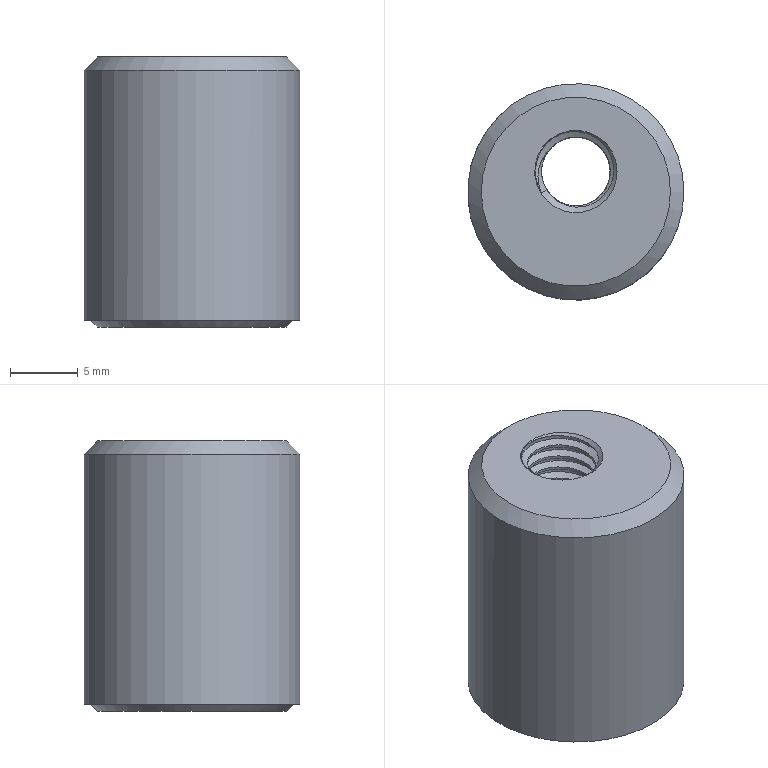Part | NX | features solid 2 | 1 solid | 21 faces | box 16.01 x 16 x 20.007 mm | volume 3058 mm3 | plane 10 | cone 5 | cylinder 4 | spline 2 | commonest cylinder face diameters 5.1 x1 6 x1 9 x1 16 x1
STEP:
#1=CARTESIAN_POINT('',(524.742,-196.458,-46.502));
#2=VERTEX_POINT('',#1);
#3=CARTESIAN_POINT('',(520.,-201.2,-46.5));
#4=VERTEX_POINT('',#3);
#5=CARTESIAN_POINT('',(522.371,-198.829,-46.501));
#6=DIRECTION('',(-0.7071,-0.7071,0.0003672));
#7=VECTOR('',#6,1000.);
#8=LINE('',#5,#7);
#9=EDGE_CURVE('',#2,#4,#8,.T.);
#10=ORIENTED_EDGE('',*,*,#9,.F.);
#11=CARTESIAN_POINT('',(523.742,-196.458,-46.502));
#12=VERTEX_POINT('',#11);
#13=CARTESIAN_POINT('',(524.242,-196.458,-46.502));
#14=DIRECTION('',(-1.,0.,0.0005193));
#15=VECTOR('',#14,1000.);
#16=LINE('',#13,#15);
#17=EDGE_CURVE('',#2,#12,#16,.T.);
#18=ORIENTED_EDGE('',*,*,#17,.T.);
#19=CARTESIAN_POINT('',(520.,-200.2,-46.5));
#20=VERTEX_POINT('',#19);
#21=CARTESIAN_POINT('',(521.871,-198.329,-46.501));
#22=DIRECTION('',(-0.7071,-0.7071,0.0003672));
#23=VECTOR('',#22,1000.);
#24=LINE('',#21,#23);
#25=EDGE_CURVE('',#12,#20,#24,.T.);
#26=ORIENTED_EDGE('',*,*,#25,.T.);
#27=CARTESIAN_POINT('',(516.154,-196.354,-46.498));
#28=VERTEX_POINT('',#27);
#29=CARTESIAN_POINT('',(517.827,-198.027,-46.499));
#30=DIRECTION('',(-0.7071,0.7071,0.0003672));
#31=VECTOR('',#30,1000.);
#32=LINE('',#29,#31);
#33=EDGE_CURVE('',#20,#28,#32,.T.);
#34=ORIENTED_EDGE('',*,*,#33,.T.);
#35=CARTESIAN_POINT('',(515.154,-196.354,-46.497));
#36=VERTEX_POINT('',#35);
#37=CARTESIAN_POINT('',(515.154,-196.354,-46.497));
#38=DIRECTION('',(1.,0.,-0.0005193));
#39=VECTOR('',#38,1000.);
#40=LINE('',#37,#39);
#41=EDGE_CURVE('',#36,#28,#40,.T.);
#42=ORIENTED_EDGE('',*,*,#41,.F.);
#43=CARTESIAN_POINT('',(517.577,-198.777,-46.499));
#44=DIRECTION('',(-0.7071,0.7071,0.0003672));
#45=VECTOR('',#44,1000.);
#46=LINE('',#43,#45);
#47=EDGE_CURVE('',#4,#36,#46,.T.);
#48=ORIENTED_EDGE('',*,*,#47,.F.);
#49=EDGE_LOOP('',(#10,#18,#26,#34,#42,#48));
#50=FACE_BOUND('',#49,.T.);
#51=CARTESIAN_POINT('',(524.5,-193.5,-46.502));
#52=VERTEX_POINT('',#51);
#53=CARTESIAN_POINT('',(520.,-193.5,-46.5));
#54=DIRECTION('',(0.0005193,0.,1.));
#55=DIRECTION('',(1.,0.,-0.0005193));
#56=AXIS2_PLACEMENT_3D('',#53,#54,#55);
#57=CIRCLE('',#56,4.5);
#58=EDGE_CURVE('',#52,#52,#57,.T.);
#59=ORIENTED_EDGE('',*,*,#58,.T.);
#60=EDGE_LOOP('',(#59));
#61=FACE_BOUND('',#60,.T.);
#62=CARTESIAN_POINT('',(526.5,-195.,-46.503));
#63=VERTEX_POINT('',#62);
#64=CARTESIAN_POINT('',(520.,-195.,-46.5));
#65=DIRECTION('',(0.0005193,0.,1.));
#66=DIRECTION('',(1.,0.,-0.0005193));
#67=AXIS2_PLACEMENT_3D('',#64,#65,#66);
#68=CIRCLE('',#67,6.5);
#69=EDGE_CURVE('',#63,#63,#68,.T.);
#70=ORIENTED_EDGE('',*,*,#69,.F.);
#71=EDGE_LOOP('',(#70));
#72=FACE_BOUND('',#71,.T.);
#73=CARTESIAN_POINT('',(520.,-195.,-46.5));
#74=DIRECTION('',(-0.0005193,0.,-1.));
#75=DIRECTION('',(1.,0.,-0.0005193));
#76=AXIS2_PLACEMENT_3D('',#73,#74,#75);
#77=PLANE('',#76);
#78=ADVANCED_FACE('',(#50,#61,#72),#77,.T.);
#79=CARTESIAN_POINT('',(512.5,-195.,-46.496));
#80=VERTEX_POINT('',#79);
#81=CARTESIAN_POINT('',(520.,-195.,-46.5));
#82=DIRECTION('',(-0.0005193,0.,-1.));
#83=DIRECTION('',(-1.,0.,0.0005193));
#84=AXIS2_PLACEMENT_3D('',#81,#82,#83);
#85=CIRCLE('',#84,7.5);
#86=EDGE_CURVE('',#80,#80,#85,.T.);
#87=ORIENTED_EDGE('',*,*,#86,.F.);
#88=EDGE_LOOP('',(#87));
#89=FACE_BOUND('',#88,.T.);
#90=CARTESIAN_POINT('',(528.,-195.,-46.504));
#91=VERTEX_POINT('',#90);
#92=CARTESIAN_POINT('',(520.,-195.,-46.5));
#93=DIRECTION('',(0.0005193,0.,1.));
#94=DIRECTION('',(1.,0.,-0.0005193));
#95=AXIS2_PLACEMENT_3D('',#92,#93,#94);
#96=CIRCLE('',#95,8.);
#97=EDGE_CURVE('',#91,#91,#96,.T.);
#98=ORIENTED_EDGE('',*,*,#97,.F.);
#99=EDGE_LOOP('',(#98));
#100=FACE_BOUND('',#99,.T.);
#101=CARTESIAN_POINT('',(520.,-195.,-46.5));
#102=DIRECTION('',(-0.0005193,0.,-1.));
#103=DIRECTION('',(1.,0.,-0.0005193));
#104=AXIS2_PLACEMENT_3D('',#101,#102,#103);
#105=PLANE('',#104);
#106=ADVANCED_FACE('',(#89,#100),#105,.T.);
#107=CARTESIAN_POINT('',(527.01,-195.,-27.004));
#108=VERTEX_POINT('',#107);
#109=CARTESIAN_POINT('',(520.01,-195.,-27.));
#110=DIRECTION('',(0.0005193,0.,1.));
#111=DIRECTION('',(1.,0.,-0.0005193));
#112=AXIS2_PLACEMENT_3D('',#109,#110,#111);
#113=CIRCLE('',#112,7.);
#114=EDGE_CURVE('',#108,#108,#113,.T.);
#115=ORIENTED_EDGE('',*,*,#114,.T.);
#116=EDGE_LOOP('',(#115));
#117=FACE_BOUND('',#116,.T.);
#118=CARTESIAN_POINT('',(523.06,-193.5,-27.002));
#119=VERTEX_POINT('',#118);
#120=CARTESIAN_POINT('',(520.01,-193.5,-27.));
#121=DIRECTION('',(-0.0005193,0.,-1.));
#122=DIRECTION('',(1.,0.,-0.0005193));
#123=AXIS2_PLACEMENT_3D('',#120,#121,#122);
#124=CIRCLE('',#123,3.05);
#125=EDGE_CURVE('',#119,#119,#124,.T.);
#126=ORIENTED_EDGE('',*,*,#125,.T.);
#127=EDGE_LOOP('',(#126));
#128=FACE_BOUND('',#127,.T.);
#129=CARTESIAN_POINT('',(520.01,-195.,-27.));
#130=DIRECTION('',(0.0005193,0.,1.));
#131=DIRECTION('',(-1.,0.,0.0005193));
#132=AXIS2_PLACEMENT_3D('',#129,#130,#131);
#133=PLANE('',#132);
#134=ADVANCED_FACE('',(#117,#128),#133,.T.);
#135=CARTESIAN_POINT('',(528.01,-195.,-28.004));
#136=VERTEX_POINT('',#135);
#137=CARTESIAN_POINT('',(520.01,-195.,-28.));
#138=DIRECTION('',(-0.0005193,0.,-1.));
#139=DIRECTION('',(1.,0.,-0.0005193));
#140=AXIS2_PLACEMENT_3D('',#137,#138,#139);
#141=CIRCLE('',#140,8.);
#142=EDGE_CURVE('',#136,#136,#141,.T.);
#143=ORIENTED_EDGE('',*,*,#142,.T.);
#144=EDGE_LOOP('',(#143));
#145=FACE_BOUND('',#144,.T.);
#146=ORIENTED_EDGE('',*,*,#97,.T.);
#147=EDGE_LOOP('',(#146));
#148=FACE_BOUND('',#147,.T.);
#149=CARTESIAN_POINT('',(520.,-195.,-46.5));
#150=DIRECTION('',(0.0005193,0.,1.));
#151=DIRECTION('',(-1.,0.,0.0005193));
#152=AXIS2_PLACEMENT_3D('',#149,#150,#151);
#153=CYLINDRICAL_SURFACE('',#152,8.);
#154=ADVANCED_FACE('',(#145,#148),#153,.T.);
#155=CARTESIAN_POINT('',(522.07,-194.996,-37.001));
#156=VERTEX_POINT('',#155);
#157=CARTESIAN_POINT('',(522.07,-192.004,-37.001));
#158=VERTEX_POINT('',#157);
#159=CARTESIAN_POINT('',(520.005,-193.5,-37.));
#160=DIRECTION('',(0.0005193,0.,1.));
#161=DIRECTION('',(1.,0.,-0.0005193));
#162=AXIS2_PLACEMENT_3D('',#159,#160,#161);
#163=CIRCLE('',#162,2.55);
#164=EDGE_CURVE('',#156,#158,#163,.T.);
#165=ORIENTED_EDGE('',*,*,#164,.F.);
#166=CARTESIAN_POINT('',(517.945,-192.004,-27.499));
#167=VERTEX_POINT('',#166);
#168=CARTESIAN_POINT('',(522.07,-194.996,-37.001));
#169=CARTESIAN_POINT('',(522.54,-194.348,-36.949));
#170=CARTESIAN_POINT('',(522.813,-192.619,-36.853));
#171=CARTESIAN_POINT('',(520.969,-190.713,-36.703));
#172=CARTESIAN_POINT('',(518.34,-191.069,-36.553));
#173=CARTESIAN_POINT('',(517.061,-193.388,-36.406));
#174=CARTESIAN_POINT('',(518.16,-195.798,-36.257));
#175=CARTESIAN_POINT('',(520.753,-196.351,-36.109));
#176=CARTESIAN_POINT('',(522.741,-194.597,-35.961));
#177=CARTESIAN_POINT('',(522.516,-191.957,-35.813));
#178=CARTESIAN_POINT('',(520.264,-190.564,-35.666));
#179=CARTESIAN_POINT('',(517.801,-191.544,-35.515));
#180=CARTESIAN_POINT('',(517.122,-194.107,-35.366));
#181=CARTESIAN_POINT('',(518.776,-196.178,-35.217));
#182=CARTESIAN_POINT('',(521.422,-196.084,-35.07));
#183=CARTESIAN_POINT('',(522.926,-193.902,-34.924));
#184=CARTESIAN_POINT('',(522.067,-191.393,-34.775));
#185=CARTESIAN_POINT('',(519.541,-190.59,-34.625));
#186=CARTESIAN_POINT('',(517.394,-192.138,-34.474));
#187=CARTESIAN_POINT('',(517.355,-194.788,-34.326));
#188=CARTESIAN_POINT('',(519.463,-196.397,-34.18));
#189=CARTESIAN_POINT('',(522.01,-195.661,-34.033));
#190=CARTESIAN_POINT('',(522.936,-193.181,-33.885));
#191=CARTESIAN_POINT('',(521.496,-190.957,-33.734));
#192=CARTESIAN_POINT('',(518.85,-190.789,-33.584));
#193=CARTESIAN_POINT('',(517.141,-192.816,-33.436));
#194=CARTESIAN_POINT('',(517.749,-195.393,-33.288));
#195=CARTESIAN_POINT('',(520.182,-196.442,-33.142));
#196=CARTESIAN_POINT('',(522.475,-195.112,-32.993));
#197=CARTESIAN_POINT('',(522.771,-192.477,-32.844));
#198=CARTESIAN_POINT('',(520.833,-190.671,-32.695));
#199=CARTESIAN_POINT('',(518.228,-191.151,-32.546));
#200=CARTESIAN_POINT('',(517.06,-193.531,-32.399));
#201=CARTESIAN_POINT('',(518.278,-195.886,-32.249));
#202=CARTESIAN_POINT('',(520.893,-196.311,-32.101));
#203=CARTESIAN_POINT('',(522.792,-194.465,-31.954));
#204=CARTESIAN_POINT('',(522.442,-191.837,-31.806));
#205=CARTESIAN_POINT('',(520.121,-190.555,-31.658));
#206=CARTESIAN_POINT('',(517.71,-191.655,-31.507));
#207=CARTESIAN_POINT('',(517.157,-194.244,-31.358));
#208=CARTESIAN_POINT('',(518.908,-196.234,-31.21));
#209=CARTESIAN_POINT('',(521.55,-196.012,-31.063));
#210=CARTESIAN_POINT('',(522.944,-193.757,-30.917));
#211=CARTESIAN_POINT('',(521.966,-191.297,-30.767));
#212=CARTESIAN_POINT('',(519.405,-190.615,-30.617));
#213=CARTESIAN_POINT('',(517.331,-192.267,-30.466));
#214=CARTESIAN_POINT('',(517.425,-194.917,-30.318));
#215=CARTESIAN_POINT('',(519.605,-196.419,-30.173));
#216=CARTESIAN_POINT('',(522.113,-195.564,-30.025));
#217=CARTESIAN_POINT('',(522.92,-193.038,-29.877));
#218=CARTESIAN_POINT('',(521.371,-190.886,-29.726));
#219=CARTESIAN_POINT('',(518.723,-190.849,-29.577));
#220=CARTESIAN_POINT('',(517.113,-192.953,-29.429));
#221=CARTESIAN_POINT('',(517.845,-195.502,-29.281));
#222=CARTESIAN_POINT('',(520.329,-196.43,-29.134));
#223=CARTESIAN_POINT('',(522.552,-194.99,-28.985));
#224=CARTESIAN_POINT('',(522.721,-192.346,-28.837));
#225=CARTESIAN_POINT('',(520.697,-190.634,-28.688));
#226=CARTESIAN_POINT('',(518.116,-191.241,-28.539));
#227=CARTESIAN_POINT('',(517.068,-193.674,-28.391));
#228=CARTESIAN_POINT('',(518.396,-195.966,-28.241));
#229=CARTESIAN_POINT('',(521.03,-196.265,-28.094));
#230=CARTESIAN_POINT('',(522.839,-194.327,-27.946));
#231=CARTESIAN_POINT('',(522.359,-191.72,-27.798));
#232=CARTESIAN_POINT('',(519.981,-190.556,-27.649));
#233=CARTESIAN_POINT('',(518.415,-191.356,-27.551));
#234=CARTESIAN_POINT('',(517.945,-192.004,-27.499));
#235=B_SPLINE_CURVE_WITH_KNOTS('',3,(#168,#169,#170,#171,#172,#173,#174,#175,#176,#177,#178,#179,#180,#181,#182,#183,#184,#185,#186,#187,#188,#189,#190,#191,#192,#193,#194,#195,#196,#197,#198,#199,#200,#201,#202,#203,#204,#205,#206,#207,#208,#209,#210,#211,#212,#213,#214,#215,#216,#217,#218,#219,#220,#221,#222,#223,#224,#225,#226,#227,#228,#229,#230,#231,#232,#233,#234),.UNSPECIFIED.,.F.,.F.,(4,1,1,1,1,1,1,1,1,1,1,1,1,1,1,1,1,1,1,1,1,1,1,1,1,1,1,1,1,1,1,1,1,1,1,1,1,1,1,1,1,1,1,1,1,1,1,1,1,1,1,1,1,1,1,1,1,1,1,1,1,1,1,1,4),(0.,0.002372,0.004743,0.007115,0.009486,0.01186,0.01423,0.0166,0.01897,0.02134,0.02372,0.02609,0.02846,0.03083,0.0332,0.03557,0.03795,0.04032,0.04269,0.04506,0.04743,0.0498,0.05217,0.05455,0.05692,0.05929,0.06166,0.06403,0.0664,0.06878,0.07115,0.07352,0.07589,0.07826,0.08063,0.083,0.08538,0.08775,0.09012,0.09249,0.09486,0.09723,0.09961,0.102,0.1043,0.1067,0.1091,0.1115,0.1138,0.1162,0.1186,0.1209,0.1233,0.1257,0.1281,0.1304,0.1328,0.1352,0.1376,0.1399,0.1423,0.1447,0.147,0.1494,0.1518),.UNSPECIFIED.);
#236=EDGE_CURVE('',#156,#167,#235,.T.);
#237=ORIENTED_EDGE('',*,*,#236,.T.);
#238=CARTESIAN_POINT('',(517.945,-194.996,-27.499));
#239=VERTEX_POINT('',#238);
#240=CARTESIAN_POINT('',(520.01,-193.5,-27.5));
#241=DIRECTION('',(0.0005193,0.,1.));
#242=DIRECTION('',(1.,0.,-0.0005193));
#243=AXIS2_PLACEMENT_3D('',#240,#241,#242);
#244=CIRCLE('',#243,2.55);
#245=EDGE_CURVE('',#167,#239,#244,.T.);
#246=ORIENTED_EDGE('',*,*,#245,.T.);
#247=CARTESIAN_POINT('',(517.945,-194.996,-27.499));
#248=CARTESIAN_POINT('',(517.476,-194.348,-27.551));
#249=CARTESIAN_POINT('',(517.202,-192.619,-27.647));
#250=CARTESIAN_POINT('',(519.047,-190.713,-27.797));
#251=CARTESIAN_POINT('',(521.675,-191.069,-27.947));
#252=CARTESIAN_POINT('',(522.954,-193.388,-28.094));
#253=CARTESIAN_POINT('',(521.855,-195.798,-28.243));
#254=CARTESIAN_POINT('',(519.263,-196.351,-28.391));
#255=CARTESIAN_POINT('',(517.274,-194.597,-28.539));
#256=CARTESIAN_POINT('',(517.499,-191.957,-28.687));
#257=CARTESIAN_POINT('',(519.751,-190.564,-28.834));
#258=CARTESIAN_POINT('',(522.214,-191.544,-28.985));
#259=CARTESIAN_POINT('',(522.894,-194.107,-29.134));
#260=CARTESIAN_POINT('',(521.239,-196.178,-29.283));
#261=CARTESIAN_POINT('',(518.593,-196.084,-29.43));
#262=CARTESIAN_POINT('',(517.089,-193.902,-29.576));
#263=CARTESIAN_POINT('',(517.948,-191.393,-29.725));
#264=CARTESIAN_POINT('',(520.474,-190.59,-29.875));
#265=CARTESIAN_POINT('',(522.622,-192.138,-30.026));
#266=CARTESIAN_POINT('',(522.66,-194.788,-30.174));
#267=CARTESIAN_POINT('',(520.552,-196.397,-30.32));
#268=CARTESIAN_POINT('',(518.005,-195.661,-30.467));
#269=CARTESIAN_POINT('',(517.079,-193.181,-30.615));
#270=CARTESIAN_POINT('',(518.519,-190.957,-30.766));
#271=CARTESIAN_POINT('',(521.165,-190.789,-30.916));
#272=CARTESIAN_POINT('',(522.875,-192.816,-31.064));
#273=CARTESIAN_POINT('',(522.266,-195.393,-31.212));
#274=CARTESIAN_POINT('',(519.834,-196.442,-31.358));
#275=CARTESIAN_POINT('',(517.54,-195.112,-31.507));
#276=CARTESIAN_POINT('',(517.244,-192.477,-31.656));
#277=CARTESIAN_POINT('',(519.182,-190.671,-31.805));
#278=CARTESIAN_POINT('',(521.787,-191.151,-31.954));
#279=CARTESIAN_POINT('',(522.955,-193.531,-32.101));
#280=CARTESIAN_POINT('',(521.738,-195.886,-32.251));
#281=CARTESIAN_POINT('',(519.122,-196.311,-32.399));
#282=CARTESIAN_POINT('',(517.223,-194.465,-32.546));
#283=CARTESIAN_POINT('',(517.573,-191.837,-32.694));
#284=CARTESIAN_POINT('',(519.894,-190.555,-32.842));
#285=CARTESIAN_POINT('',(522.305,-191.655,-32.993));
#286=CARTESIAN_POINT('',(522.858,-194.244,-33.142));
#287=CARTESIAN_POINT('',(521.108,-196.234,-33.29));
#288=CARTESIAN_POINT('',(518.465,-196.012,-33.437));
#289=CARTESIAN_POINT('',(517.071,-193.757,-33.583));
#290=CARTESIAN_POINT('',(518.05,-191.297,-33.733));
#291=CARTESIAN_POINT('',(520.61,-190.615,-33.883));
#292=CARTESIAN_POINT('',(522.684,-192.267,-34.034));
#293=CARTESIAN_POINT('',(522.591,-194.917,-34.182));
#294=CARTESIAN_POINT('',(520.41,-196.419,-34.327));
#295=CARTESIAN_POINT('',(517.902,-195.564,-34.475));
#296=CARTESIAN_POINT('',(517.095,-193.038,-34.623));
#297=CARTESIAN_POINT('',(518.645,-190.886,-34.774));
#298=CARTESIAN_POINT('',(521.292,-190.849,-34.923));
#299=CARTESIAN_POINT('',(522.902,-192.953,-35.071));
#300=CARTESIAN_POINT('',(522.17,-195.502,-35.219));
#301=CARTESIAN_POINT('',(519.686,-196.43,-35.366));
#302=CARTESIAN_POINT('',(517.464,-194.99,-35.515));
#303=CARTESIAN_POINT('',(517.294,-192.346,-35.663));
#304=CARTESIAN_POINT('',(519.318,-190.634,-35.812));
#305=CARTESIAN_POINT('',(521.899,-191.241,-35.961));
#306=CARTESIAN_POINT('',(522.947,-193.674,-36.109));
#307=CARTESIAN_POINT('',(521.62,-195.966,-36.259));
#308=CARTESIAN_POINT('',(518.985,-196.265,-36.406));
#309=CARTESIAN_POINT('',(517.176,-194.327,-36.554));
#310=CARTESIAN_POINT('',(517.656,-191.72,-36.702));
#311=CARTESIAN_POINT('',(520.035,-190.556,-36.851));
#312=CARTESIAN_POINT('',(521.601,-191.356,-36.949));
#313=CARTESIAN_POINT('',(522.07,-192.004,-37.001));
#314=B_SPLINE_CURVE_WITH_KNOTS('',3,(#247,#248,#249,#250,#251,#252,#253,#254,#255,#256,#257,#258,#259,#260,#261,#262,#263,#264,#265,#266,#267,#268,#269,#270,#271,#272,#273,#274,#275,#276,#277,#278,#279,#280,#281,#282,#283,#284,#285,#286,#287,#288,#289,#290,#291,#292,#293,#294,#295,#296,#297,#298,#299,#300,#301,#302,#303,#304,#305,#306,#307,#308,#309,#310,#311,#312,#313),.UNSPECIFIED.,.F.,.F.,(4,1,1,1,1,1,1,1,1,1,1,1,1,1,1,1,1,1,1,1,1,1,1,1,1,1,1,1,1,1,1,1,1,1,1,1,1,1,1,1,1,1,1,1,1,1,1,1,1,1,1,1,1,1,1,1,1,1,1,1,1,1,1,1,4),(0.,0.002372,0.004743,0.007115,0.009486,0.01186,0.01423,0.0166,0.01897,0.02134,0.02372,0.02609,0.02846,0.03083,0.0332,0.03557,0.03795,0.04032,0.04269,0.04506,0.04743,0.0498,0.05217,0.05455,0.05692,0.05929,0.06166,0.06403,0.0664,0.06878,0.07115,0.07352,0.07589,0.07826,0.08063,0.083,0.08538,0.08775,0.09012,0.09249,0.09486,0.09723,0.09961,0.102,0.1043,0.1067,0.1091,0.1115,0.1138,0.1162,0.1186,0.1209,0.1233,0.1257,0.1281,0.1304,0.1328,0.1352,0.1376,0.1399,0.1423,0.1447,0.147,0.1494,0.1518),.UNSPECIFIED.);
#315=EDGE_CURVE('',#239,#158,#314,.T.);
#316=ORIENTED_EDGE('',*,*,#315,.T.);
#317=EDGE_LOOP('',(#165,#237,#246,#316));
#318=FACE_BOUND('',#317,.T.);
#319=CARTESIAN_POINT('',(520.011,-193.5,-26.5));
#320=DIRECTION('',(0.0005193,0.,1.));
#321=DIRECTION('',(-1.,0.,0.0005193));
#322=AXIS2_PLACEMENT_3D('',#319,#320,#321);
#323=CYLINDRICAL_SURFACE('',#322,2.55);
#324=ADVANCED_FACE('',(#318),#323,.F.);
#325=CARTESIAN_POINT('',(518.102,-191.181,-36.999));
#326=VERTEX_POINT('',#325);
#327=CARTESIAN_POINT('',(518.102,-195.819,-36.999));
#328=VERTEX_POINT('',#327);
#329=CARTESIAN_POINT('',(520.005,-193.5,-37.));
#330=DIRECTION('',(0.0005193,0.,1.));
#331=DIRECTION('',(1.,0.,-0.0005193));
#332=AXIS2_PLACEMENT_3D('',#329,#330,#331);
#333=CIRCLE('',#332,3.);
#334=EDGE_CURVE('',#326,#328,#333,.T.);
#335=ORIENTED_EDGE('',*,*,#334,.T.);
#336=CARTESIAN_POINT('',(518.102,-195.819,-36.999));
#337=CARTESIAN_POINT('',(518.737,-196.246,-36.999));
#338=CARTESIAN_POINT('',(520.325,-196.591,-37.));
#339=CARTESIAN_POINT('',(521.693,-195.663,-37.001));
#340=CARTESIAN_POINT('',(522.07,-194.996,-37.001));
#341=B_SPLINE_CURVE_WITH_KNOTS('',3,(#336,#337,#338,#339,#340),.UNSPECIFIED.,.F.,.F.,(4,1,4),(0.,0.002262,0.004525),.UNSPECIFIED.);
#342=EDGE_CURVE('',#328,#156,#341,.T.);
#343=ORIENTED_EDGE('',*,*,#342,.T.);
#344=ORIENTED_EDGE('',*,*,#164,.T.);
#345=CARTESIAN_POINT('',(522.07,-192.004,-37.001));
#346=CARTESIAN_POINT('',(521.693,-191.338,-37.001));
#347=CARTESIAN_POINT('',(520.327,-190.409,-37.));
#348=CARTESIAN_POINT('',(518.737,-190.754,-36.999));
#349=CARTESIAN_POINT('',(518.102,-191.181,-36.999));
#350=B_SPLINE_CURVE_WITH_KNOTS('',3,(#345,#346,#347,#348,#349),.UNSPECIFIED.,.F.,.F.,(4,1,4),(0.,0.002264,0.004528),.UNSPECIFIED.);
#351=EDGE_CURVE('',#158,#326,#350,.T.);
#352=ORIENTED_EDGE('',*,*,#351,.T.);
#353=EDGE_LOOP('',(#335,#343,#344,#352));
#354=FACE_BOUND('',#353,.T.);
#355=CARTESIAN_POINT('',(524.505,-193.5,-37.002));
#356=VERTEX_POINT('',#355);
#357=CARTESIAN_POINT('',(520.005,-193.5,-37.));
#358=DIRECTION('',(0.0005193,0.,1.));
#359=DIRECTION('',(1.,0.,-0.0005193));
#360=AXIS2_PLACEMENT_3D('',#357,#358,#359);
#361=CIRCLE('',#360,4.5);
#362=EDGE_CURVE('',#356,#356,#361,.T.);
#363=ORIENTED_EDGE('',*,*,#362,.F.);
#364=EDGE_LOOP('',(#363));
#365=FACE_BOUND('',#364,.T.);
#366=CARTESIAN_POINT('',(520.005,-193.5,-37.));
#367=DIRECTION('',(0.0005193,0.,1.));
#368=DIRECTION('',(-1.,0.,0.0005193));
#369=AXIS2_PLACEMENT_3D('',#366,#367,#368);
#370=PLANE('',#369);
#371=ADVANCED_FACE('',(#354,#365),#370,.F.);
#372=ORIENTED_EDGE('',*,*,#362,.T.);
#373=EDGE_LOOP('',(#372));
#374=FACE_BOUND('',#373,.T.);
#375=ORIENTED_EDGE('',*,*,#58,.F.);
#376=EDGE_LOOP('',(#375));
#377=FACE_BOUND('',#376,.T.);
#378=CARTESIAN_POINT('',(520.,-193.5,-46.5));
#379=DIRECTION('',(0.0005193,0.,1.));
#380=DIRECTION('',(-1.,0.,0.0005193));
#381=AXIS2_PLACEMENT_3D('',#378,#379,#380);
#382=CYLINDRICAL_SURFACE('',#381,4.5);
#383=ADVANCED_FACE('',(#374,#377),#382,.F.);
#384=CARTESIAN_POINT('',(517.476,-195.105,-27.049));
#385=VERTEX_POINT('',#384);
#386=CARTESIAN_POINT('',(517.476,-195.105,-27.049));
#387=CARTESIAN_POINT('',(516.992,-194.09,-27.183));
#388=CARTESIAN_POINT('',(517.157,-192.801,-27.328));
#389=CARTESIAN_POINT('',(517.945,-192.004,-27.499));
#390=B_SPLINE_CURVE_WITH_KNOTS('',3,(#386,#387,#388,#389),.UNSPECIFIED.,.F.,.F.,(4,4),(0.,0.003348),.UNSPECIFIED.);
#391=EDGE_CURVE('',#385,#167,#390,.T.);
#392=ORIENTED_EDGE('',*,*,#391,.F.);
#393=CARTESIAN_POINT('',(518.893,-190.716,-27.049));
#394=VERTEX_POINT('',#393);
#395=CARTESIAN_POINT('',(520.01,-193.5,-27.05));
#396=DIRECTION('',(0.0005193,0.,1.));
#397=DIRECTION('',(1.,0.,-0.0005193));
#398=AXIS2_PLACEMENT_3D('',#395,#396,#397);
#399=CIRCLE('',#398,3.);
#400=EDGE_CURVE('',#394,#385,#399,.T.);
#401=ORIENTED_EDGE('',*,*,#400,.F.);
#402=CARTESIAN_POINT('',(517.945,-194.996,-27.499));
#403=CARTESIAN_POINT('',(518.523,-195.866,-27.456));
#404=CARTESIAN_POINT('',(520.792,-196.737,-27.381));
#405=CARTESIAN_POINT('',(523.371,-194.165,-27.266));
#406=CARTESIAN_POINT('',(522.19,-190.766,-27.155));
#407=CARTESIAN_POINT('',(519.873,-190.36,-27.085));
#408=CARTESIAN_POINT('',(518.893,-190.716,-27.049));
#409=B_SPLINE_CURVE_WITH_KNOTS('',3,(#402,#403,#404,#405,#406,#407,#408),.UNSPECIFIED.,.F.,.F.,(4,1,1,1,4),(0.,0.00309,0.006179,0.009269,0.01236),.UNSPECIFIED.);
#410=EDGE_CURVE('',#239,#394,#409,.T.);
#411=ORIENTED_EDGE('',*,*,#410,.F.);
#412=ORIENTED_EDGE('',*,*,#245,.F.);
#413=EDGE_LOOP('',(#392,#401,#411,#412));
#414=FACE_BOUND('',#413,.T.);
#415=ORIENTED_EDGE('',*,*,#125,.F.);
#416=EDGE_LOOP('',(#415));
#417=FACE_BOUND('',#416,.T.);
#418=CARTESIAN_POINT('',(520.01,-193.5,-27.5));
#419=DIRECTION('',(0.0005193,0.,1.));
#420=DIRECTION('',(-1.,0.,0.0005193));
#421=AXIS2_PLACEMENT_3D('',#418,#419,#420);
#422=CONICAL_SURFACE('',#421,2.55,0.7854);
#423=ADVANCED_FACE('',(#414,#417),#422,.F.);
#424=ORIENTED_EDGE('',*,*,#400,.T.);
#425=CARTESIAN_POINT('',(517.476,-195.105,-27.049));
#426=CARTESIAN_POINT('',(516.948,-194.271,-27.099));
#427=CARTESIAN_POINT('',(516.793,-192.097,-27.203));
#428=CARTESIAN_POINT('',(519.373,-190.04,-27.361));
#429=CARTESIAN_POINT('',(522.52,-191.038,-27.519));
#430=CARTESIAN_POINT('',(523.455,-194.202,-27.674));
#431=CARTESIAN_POINT('',(521.356,-196.749,-27.827));
#432=CARTESIAN_POINT('',(518.071,-196.433,-27.982));
#433=CARTESIAN_POINT('',(516.494,-193.534,-28.139));
#434=CARTESIAN_POINT('',(518.014,-190.606,-28.293));
#435=CARTESIAN_POINT('',(521.29,-190.226,-28.449));
#436=CARTESIAN_POINT('',(523.439,-192.728,-28.606));
#437=CARTESIAN_POINT('',(522.57,-195.91,-28.763));
#438=CARTESIAN_POINT('',(519.445,-196.971,-28.916));
#439=CARTESIAN_POINT('',(516.817,-194.975,-29.068));
#440=CARTESIAN_POINT('',(517.001,-191.68,-29.224));
#441=CARTESIAN_POINT('',(519.834,-189.988,-29.384));
#442=CARTESIAN_POINT('',(522.822,-191.39,-29.539));
#443=CARTESIAN_POINT('',(523.332,-194.65,-29.694));
#444=CARTESIAN_POINT('',(520.916,-196.897,-29.848));
#445=CARTESIAN_POINT('',(517.703,-196.154,-30.004));
#446=CARTESIAN_POINT('',(516.519,-193.075,-30.159));
#447=CARTESIAN_POINT('',(518.408,-190.37,-30.313));
#448=CARTESIAN_POINT('',(521.707,-190.421,-30.47));
#449=CARTESIAN_POINT('',(523.511,-193.185,-30.629));
#450=CARTESIAN_POINT('',(522.229,-196.226,-30.783));
#451=CARTESIAN_POINT('',(518.992,-196.866,-30.936));
#452=CARTESIAN_POINT('',(516.65,-194.541,-31.09));
#453=CARTESIAN_POINT('',(517.266,-191.3,-31.247));
#454=CARTESIAN_POINT('',(520.295,-189.996,-31.405));
#455=CARTESIAN_POINT('',(523.072,-191.776,-31.559));
#456=CARTESIAN_POINT('',(523.152,-195.074,-31.714));
#457=CARTESIAN_POINT('',(520.463,-196.987,-31.871));
#458=CARTESIAN_POINT('',(517.373,-195.828,-32.025));
#459=CARTESIAN_POINT('',(516.604,-192.619,-32.178));
#460=CARTESIAN_POINT('',(518.833,-190.186,-32.334));
#461=CARTESIAN_POINT('',(522.097,-190.672,-32.492));
#462=CARTESIAN_POINT('',(523.52,-193.648,-32.651));
#463=CARTESIAN_POINT('',(521.851,-196.493,-32.802));
#464=CARTESIAN_POINT('',(518.56,-196.704,-32.956));
#465=CARTESIAN_POINT('',(516.542,-194.094,-33.112));
#466=CARTESIAN_POINT('',(517.575,-190.961,-33.268));
#467=CARTESIAN_POINT('',(520.751,-190.063,-33.425));
#468=CARTESIAN_POINT('',(523.271,-192.194,-33.58));
#469=CARTESIAN_POINT('',(522.916,-195.474,-33.736));
#470=CARTESIAN_POINT('',(519.999,-197.016,-33.893));
#471=CARTESIAN_POINT('',(517.089,-195.461,-34.044));
#472=CARTESIAN_POINT('',(516.748,-192.18,-34.198));
#473=CARTESIAN_POINT('',(519.275,-190.061,-34.356));
#474=CARTESIAN_POINT('',(522.447,-190.969,-34.515));
#475=CARTESIAN_POINT('',(523.47,-194.106,-34.67));
#476=CARTESIAN_POINT('',(521.443,-196.71,-34.823));
#477=CARTESIAN_POINT('',(518.15,-196.486,-34.977));
#478=CARTESIAN_POINT('',(516.492,-193.633,-35.134));
#479=CARTESIAN_POINT('',(517.93,-190.662,-35.289));
#480=CARTESIAN_POINT('',(521.196,-190.191,-35.445));
#481=CARTESIAN_POINT('',(523.413,-192.634,-35.602));
#482=CARTESIAN_POINT('',(522.632,-195.838,-35.758));
#483=CARTESIAN_POINT('',(519.539,-196.985,-35.912));
#484=CARTESIAN_POINT('',(516.856,-195.063,-36.064));
#485=CARTESIAN_POINT('',(516.947,-191.765,-36.22));
#486=CARTESIAN_POINT('',(519.732,-189.995,-36.379));
#487=CARTESIAN_POINT('',(522.758,-191.312,-36.535));
#488=CARTESIAN_POINT('',(523.361,-194.558,-36.689));
#489=CARTESIAN_POINT('',(521.,-196.866,-36.845));
#490=CARTESIAN_POINT('',(518.864,-196.445,-36.945));
#491=CARTESIAN_POINT('',(518.102,-195.819,-36.999));
#492=B_SPLINE_CURVE_WITH_KNOTS('',3,(#425,#426,#427,#428,#429,#430,#431,#432,#433,#434,#435,#436,#437,#438,#439,#440,#441,#442,#443,#444,#445,#446,#447,#448,#449,#450,#451,#452,#453,#454,#455,#456,#457,#458,#459,#460,#461,#462,#463,#464,#465,#466,#467,#468,#469,#470,#471,#472,#473,#474,#475,#476,#477,#478,#479,#480,#481,#482,#483,#484,#485,#486,#487,#488,#489,#490,#491),.UNSPECIFIED.,.F.,.F.,(4,1,1,1,1,1,1,1,1,1,1,1,1,1,1,1,1,1,1,1,1,1,1,1,1,1,1,1,1,1,1,1,1,1,1,1,1,1,1,1,1,1,1,1,1,1,1,1,1,1,1,1,1,1,1,1,1,1,1,1,1,1,1,1,4),(0.,0.002923,0.005846,0.008769,0.01169,0.01461,0.01754,0.02046,0.02338,0.02631,0.02923,0.03215,0.03508,0.038,0.04092,0.04384,0.04677,0.04969,0.05261,0.05554,0.05846,0.06138,0.06431,0.06723,0.07015,0.07307,0.076,0.07892,0.08184,0.08477,0.08769,0.09061,0.09353,0.09646,0.09938,0.1023,0.1052,0.1081,0.1111,0.114,0.1169,0.1198,0.1228,0.1257,0.1286,0.1315,0.1345,0.1374,0.1403,0.1432,0.1461,0.1491,0.152,0.1549,0.1578,0.1608,0.1637,0.1666,0.1695,0.1725,0.1754,0.1783,0.1812,0.1841,0.1871),.UNSPECIFIED.);
#493=EDGE_CURVE('',#385,#328,#492,.T.);
#494=ORIENTED_EDGE('',*,*,#493,.T.);
#495=ORIENTED_EDGE('',*,*,#334,.F.);
#496=CARTESIAN_POINT('',(518.102,-191.181,-36.999));
#497=CARTESIAN_POINT('',(517.34,-191.807,-36.944));
#498=CARTESIAN_POINT('',(516.51,-193.823,-36.843));
#499=CARTESIAN_POINT('',(518.316,-196.586,-36.69));
#500=CARTESIAN_POINT('',(521.619,-196.624,-36.536));
#501=CARTESIAN_POINT('',(523.498,-193.911,-36.379));
#502=CARTESIAN_POINT('',(522.3,-190.835,-36.223));
#503=CARTESIAN_POINT('',(519.08,-190.107,-36.067));
#504=CARTESIAN_POINT('',(516.676,-192.369,-35.911));
#505=CARTESIAN_POINT('',(517.206,-195.627,-35.755));
#506=CARTESIAN_POINT('',(520.201,-197.011,-35.599));
#507=CARTESIAN_POINT('',(523.024,-195.303,-35.448));
#508=CARTESIAN_POINT('',(523.19,-192.008,-35.293));
#509=CARTESIAN_POINT('',(520.551,-190.026,-35.134));
#510=CARTESIAN_POINT('',(517.431,-191.105,-34.977));
#511=CARTESIAN_POINT('',(516.581,-194.295,-34.822));
#512=CARTESIAN_POINT('',(518.749,-196.784,-34.669));
#513=CARTESIAN_POINT('',(522.025,-196.379,-34.514));
#514=CARTESIAN_POINT('',(523.522,-193.438,-34.357));
#515=CARTESIAN_POINT('',(521.922,-190.552,-34.203));
#516=CARTESIAN_POINT('',(518.636,-190.262,-34.047));
#517=CARTESIAN_POINT('',(516.556,-192.824,-33.889));
#518=CARTESIAN_POINT('',(517.515,-195.981,-33.733));
#519=CARTESIAN_POINT('',(520.67,-196.953,-33.58));
#520=CARTESIAN_POINT('',(523.24,-194.882,-33.427));
#521=CARTESIAN_POINT('',(522.962,-191.593,-33.271));
#522=CARTESIAN_POINT('',(520.079,-189.984,-33.111));
#523=CARTESIAN_POINT('',(517.134,-191.473,-32.956));
#524=CARTESIAN_POINT('',(516.72,-194.748,-32.802));
#525=CARTESIAN_POINT('',(519.201,-196.922,-32.647));
#526=CARTESIAN_POINT('',(522.392,-196.084,-32.491));
#527=CARTESIAN_POINT('',(523.484,-192.97,-32.337));
#528=CARTESIAN_POINT('',(521.513,-190.322,-32.182));
#529=CARTESIAN_POINT('',(518.215,-190.475,-32.025));
#530=CARTESIAN_POINT('',(516.497,-193.293,-31.866));
#531=CARTESIAN_POINT('',(517.873,-196.294,-31.712));
#532=CARTESIAN_POINT('',(521.13,-196.833,-31.56));
#533=CARTESIAN_POINT('',(523.398,-194.435,-31.405));
#534=CARTESIAN_POINT('',(522.68,-191.215,-31.248));
#535=CARTESIAN_POINT('',(519.61,-190.007,-31.09));
#536=CARTESIAN_POINT('',(516.89,-191.875,-30.936));
#537=CARTESIAN_POINT('',(516.917,-195.175,-30.78));
#538=CARTESIAN_POINT('',(519.667,-197.,-30.624));
#539=CARTESIAN_POINT('',(522.719,-195.741,-30.471));
#540=CARTESIAN_POINT('',(523.382,-192.507,-30.317));
#541=CARTESIAN_POINT('',(521.072,-190.148,-30.16));
#542=CARTESIAN_POINT('',(517.826,-190.743,-30.002));
#543=CARTESIAN_POINT('',(516.503,-193.766,-29.844));
#544=CARTESIAN_POINT('',(518.267,-196.554,-29.692));
#545=CARTESIAN_POINT('',(521.565,-196.653,-29.539));
#546=CARTESIAN_POINT('',(523.493,-193.975,-29.382));
#547=CARTESIAN_POINT('',(522.352,-190.878,-29.226));
#548=CARTESIAN_POINT('',(519.146,-190.091,-29.07));
#549=CARTESIAN_POINT('',(516.701,-192.309,-28.914));
#550=CARTESIAN_POINT('',(517.171,-195.576,-28.758));
#551=CARTESIAN_POINT('',(520.142,-197.014,-28.602));
#552=CARTESIAN_POINT('',(522.996,-195.356,-28.451));
#553=CARTESIAN_POINT('',(523.219,-192.064,-28.296));
#554=CARTESIAN_POINT('',(520.617,-190.037,-28.137));
#555=CARTESIAN_POINT('',(517.479,-191.059,-27.98));
#556=CARTESIAN_POINT('',(516.571,-194.232,-27.825));
#557=CARTESIAN_POINT('',(518.693,-196.76,-27.672));
#558=CARTESIAN_POINT('',(521.975,-196.416,-27.517));
#559=CARTESIAN_POINT('',(523.529,-193.501,-27.36));
#560=CARTESIAN_POINT('',(521.97,-190.589,-27.206));
#561=CARTESIAN_POINT('',(519.808,-190.348,-27.102));
#562=CARTESIAN_POINT('',(518.893,-190.716,-27.049));
#563=B_SPLINE_CURVE_WITH_KNOTS('',3,(#496,#497,#498,#499,#500,#501,#502,#503,#504,#505,#506,#507,#508,#509,#510,#511,#512,#513,#514,#515,#516,#517,#518,#519,#520,#521,#522,#523,#524,#525,#526,#527,#528,#529,#530,#531,#532,#533,#534,#535,#536,#537,#538,#539,#540,#541,#542,#543,#544,#545,#546,#547,#548,#549,#550,#551,#552,#553,#554,#555,#556,#557,#558,#559,#560,#561,#562),.UNSPECIFIED.,.F.,.F.,(4,1,1,1,1,1,1,1,1,1,1,1,1,1,1,1,1,1,1,1,1,1,1,1,1,1,1,1,1,1,1,1,1,1,1,1,1,1,1,1,1,1,1,1,1,1,1,1,1,1,1,1,1,1,1,1,1,1,1,1,1,1,1,1,4),(0.,0.002924,0.005847,0.008771,0.01169,0.01462,0.01754,0.02047,0.02339,0.02631,0.02924,0.03216,0.03508,0.03801,0.04093,0.04385,0.04678,0.0497,0.05263,0.05555,0.05847,0.0614,0.06432,0.06724,0.07017,0.07309,0.07601,0.07894,0.08186,0.08478,0.08771,0.09063,0.09356,0.09648,0.0994,0.1023,0.1053,0.1082,0.1111,0.114,0.1169,0.1199,0.1228,0.1257,0.1286,0.1316,0.1345,0.1374,0.1403,0.1433,0.1462,0.1491,0.152,0.155,0.1579,0.1608,0.1637,0.1666,0.1696,0.1725,0.1754,0.1783,0.1813,0.1842,0.1871),.UNSPECIFIED.);
#564=EDGE_CURVE('',#326,#394,#563,.T.);
#565=ORIENTED_EDGE('',*,*,#564,.T.);
#566=EDGE_LOOP('',(#424,#494,#495,#565));
#567=FACE_BOUND('',#566,.T.);
#568=CARTESIAN_POINT('',(520.011,-193.5,-26.5));
#569=DIRECTION('',(-0.0005193,0.,-1.));
#570=DIRECTION('',(1.,0.,-0.0005193));
#571=AXIS2_PLACEMENT_3D('',#568,#569,#570);
#572=CYLINDRICAL_SURFACE('',#571,3.);
#573=ADVANCED_FACE('',(#567),#572,.F.);
#574=ORIENTED_EDGE('',*,*,#391,.T.);
#575=ORIENTED_EDGE('',*,*,#236,.F.);
#576=ORIENTED_EDGE('',*,*,#342,.F.);
#577=ORIENTED_EDGE('',*,*,#493,.F.);
#578=EDGE_LOOP('',(#574,#575,#576,#577));
#579=FACE_BOUND('',#578,.T.);
#580=CARTESIAN_POINT('',(518.508,-195.553,-27.253));
#581=CARTESIAN_POINT('',(518.402,-195.477,-27.261));
#582=CARTESIAN_POINT('',(517.794,-194.96,-27.311));
#583=CARTESIAN_POINT('',(517.188,-193.5,-27.402));
#584=CARTESIAN_POINT('',(518.016,-191.506,-27.527));
#585=CARTESIAN_POINT('',(520.01,-190.678,-27.653));
#586=CARTESIAN_POINT('',(522.004,-191.506,-27.78));
#587=CARTESIAN_POINT('',(522.832,-193.5,-27.905));
#588=CARTESIAN_POINT('',(522.004,-195.494,-28.03));
#589=CARTESIAN_POINT('',(520.01,-196.322,-28.153));
#590=CARTESIAN_POINT('',(518.015,-195.494,-28.277));
#591=CARTESIAN_POINT('',(517.188,-193.5,-28.402));
#592=CARTESIAN_POINT('',(518.015,-191.506,-28.527));
#593=CARTESIAN_POINT('',(520.01,-190.678,-28.653));
#594=CARTESIAN_POINT('',(522.004,-191.506,-28.78));
#595=CARTESIAN_POINT('',(522.831,-193.5,-28.905));
#596=CARTESIAN_POINT('',(522.004,-195.494,-29.03));
#597=CARTESIAN_POINT('',(520.009,-196.322,-29.153));
#598=CARTESIAN_POINT('',(518.015,-195.494,-29.277));
#599=CARTESIAN_POINT('',(517.187,-193.5,-29.402));
#600=CARTESIAN_POINT('',(518.015,-191.506,-29.527));
#601=CARTESIAN_POINT('',(520.009,-190.678,-29.653));
#602=CARTESIAN_POINT('',(522.003,-191.506,-29.78));
#603=CARTESIAN_POINT('',(522.831,-193.5,-29.905));
#604=CARTESIAN_POINT('',(522.003,-195.494,-30.03));
#605=CARTESIAN_POINT('',(520.009,-196.322,-30.153));
#606=CARTESIAN_POINT('',(518.014,-195.494,-30.277));
#607=CARTESIAN_POINT('',(517.187,-193.5,-30.402));
#608=CARTESIAN_POINT('',(518.014,-191.506,-30.527));
#609=CARTESIAN_POINT('',(520.008,-190.678,-30.653));
#610=CARTESIAN_POINT('',(522.003,-191.506,-30.78));
#611=CARTESIAN_POINT('',(522.83,-193.5,-30.905));
#612=CARTESIAN_POINT('',(522.003,-195.494,-31.03));
#613=CARTESIAN_POINT('',(520.008,-196.322,-31.153));
#614=CARTESIAN_POINT('',(518.014,-195.494,-31.277));
#615=CARTESIAN_POINT('',(517.186,-193.5,-31.402));
#616=CARTESIAN_POINT('',(518.014,-191.506,-31.527));
#617=CARTESIAN_POINT('',(520.008,-190.678,-31.653));
#618=CARTESIAN_POINT('',(522.002,-191.506,-31.78));
#619=CARTESIAN_POINT('',(522.83,-193.5,-31.905));
#620=CARTESIAN_POINT('',(522.002,-195.494,-32.03));
#621=CARTESIAN_POINT('',(520.008,-196.322,-32.153));
#622=CARTESIAN_POINT('',(518.013,-195.494,-32.277));
#623=CARTESIAN_POINT('',(517.186,-193.5,-32.402));
#624=CARTESIAN_POINT('',(518.013,-191.506,-32.527));
#625=CARTESIAN_POINT('',(520.007,-190.678,-32.653));
#626=CARTESIAN_POINT('',(522.002,-191.506,-32.78));
#627=CARTESIAN_POINT('',(522.829,-193.5,-32.905));
#628=CARTESIAN_POINT('',(522.002,-195.494,-33.03));
#629=CARTESIAN_POINT('',(520.007,-196.322,-33.153));
#630=CARTESIAN_POINT('',(518.013,-195.494,-33.277));
#631=CARTESIAN_POINT('',(517.185,-193.5,-33.402));
#632=CARTESIAN_POINT('',(518.013,-191.506,-33.527));
#633=CARTESIAN_POINT('',(520.007,-190.678,-33.653));
#634=CARTESIAN_POINT('',(522.001,-191.506,-33.78));
#635=CARTESIAN_POINT('',(522.829,-193.5,-33.905));
#636=CARTESIAN_POINT('',(522.001,-195.494,-34.03));
#637=CARTESIAN_POINT('',(520.007,-196.322,-34.153));
#638=CARTESIAN_POINT('',(518.012,-195.494,-34.277));
#639=CARTESIAN_POINT('',(517.185,-193.5,-34.402));
#640=CARTESIAN_POINT('',(518.012,-191.506,-34.527));
#641=CARTESIAN_POINT('',(520.006,-190.678,-34.653));
#642=CARTESIAN_POINT('',(522.001,-191.506,-34.78));
#643=CARTESIAN_POINT('',(522.828,-193.5,-34.905));
#644=CARTESIAN_POINT('',(522.001,-195.494,-35.03));
#645=CARTESIAN_POINT('',(520.006,-196.322,-35.153));
#646=CARTESIAN_POINT('',(518.012,-195.494,-35.277));
#647=CARTESIAN_POINT('',(517.184,-193.5,-35.402));
#648=CARTESIAN_POINT('',(518.012,-191.506,-35.527));
#649=CARTESIAN_POINT('',(520.006,-190.678,-35.653));
#650=CARTESIAN_POINT('',(522.,-191.506,-35.78));
#651=CARTESIAN_POINT('',(522.828,-193.5,-35.905));
#652=CARTESIAN_POINT('',(522.,-195.494,-36.03));
#653=CARTESIAN_POINT('',(520.006,-196.322,-36.153));
#654=CARTESIAN_POINT('',(518.011,-195.494,-36.277));
#655=CARTESIAN_POINT('',(517.184,-193.5,-36.402));
#656=CARTESIAN_POINT('',(518.011,-191.506,-36.527));
#657=CARTESIAN_POINT('',(520.005,-190.678,-36.653));
#658=CARTESIAN_POINT('',(522.,-191.506,-36.78));
#659=CARTESIAN_POINT('',(522.827,-193.5,-36.905));
#660=CARTESIAN_POINT('',(522.,-195.494,-37.03));
#661=CARTESIAN_POINT('',(520.005,-196.322,-37.153));
#662=CARTESIAN_POINT('',(518.441,-195.673,-37.251));
#663=CARTESIAN_POINT('',(517.898,-194.944,-37.307));
#664=CARTESIAN_POINT('',(517.784,-194.739,-37.321));
#665=CARTESIAN_POINT('',(518.236,-195.926,-26.987));
#666=CARTESIAN_POINT('',(518.111,-195.835,-26.995));
#667=CARTESIAN_POINT('',(517.392,-195.225,-27.044));
#668=CARTESIAN_POINT('',(516.677,-193.5,-27.135));
#669=CARTESIAN_POINT('',(517.654,-191.144,-27.261));
#670=CARTESIAN_POINT('',(520.01,-190.166,-27.387));
#671=CARTESIAN_POINT('',(522.366,-191.144,-27.513));
#672=CARTESIAN_POINT('',(523.344,-193.5,-27.639));
#673=CARTESIAN_POINT('',(522.366,-195.856,-27.763));
#674=CARTESIAN_POINT('',(520.01,-196.834,-27.887));
#675=CARTESIAN_POINT('',(517.654,-195.856,-28.011));
#676=CARTESIAN_POINT('',(516.676,-193.5,-28.135));
#677=CARTESIAN_POINT('',(517.654,-191.144,-28.261));
#678=CARTESIAN_POINT('',(520.01,-190.166,-28.387));
#679=CARTESIAN_POINT('',(522.366,-191.144,-28.513));
#680=CARTESIAN_POINT('',(523.343,-193.5,-28.639));
#681=CARTESIAN_POINT('',(522.365,-195.856,-28.763));
#682=CARTESIAN_POINT('',(520.009,-196.834,-28.887));
#683=CARTESIAN_POINT('',(517.653,-195.856,-29.011));
#684=CARTESIAN_POINT('',(516.676,-193.5,-29.135));
#685=CARTESIAN_POINT('',(517.653,-191.144,-29.261));
#686=CARTESIAN_POINT('',(520.009,-190.166,-29.387));
#687=CARTESIAN_POINT('',(522.365,-191.144,-29.513));
#688=CARTESIAN_POINT('',(523.343,-193.5,-29.639));
#689=CARTESIAN_POINT('',(522.365,-195.856,-29.763));
#690=CARTESIAN_POINT('',(520.009,-196.834,-29.887));
#691=CARTESIAN_POINT('',(517.653,-195.856,-30.011));
#692=CARTESIAN_POINT('',(516.675,-193.5,-30.135));
#693=CARTESIAN_POINT('',(517.653,-191.144,-30.261));
#694=CARTESIAN_POINT('',(520.009,-190.166,-30.387));
#695=CARTESIAN_POINT('',(522.364,-191.144,-30.513));
#696=CARTESIAN_POINT('',(523.342,-193.5,-30.639));
#697=CARTESIAN_POINT('',(522.364,-195.856,-30.763));
#698=CARTESIAN_POINT('',(520.008,-196.834,-30.887));
#699=CARTESIAN_POINT('',(517.652,-195.856,-31.011));
#700=CARTESIAN_POINT('',(516.675,-193.5,-31.135));
#701=CARTESIAN_POINT('',(517.652,-191.144,-31.261));
#702=CARTESIAN_POINT('',(520.008,-190.166,-31.387));
#703=CARTESIAN_POINT('',(522.364,-191.144,-31.513));
#704=CARTESIAN_POINT('',(523.341,-193.5,-31.639));
#705=CARTESIAN_POINT('',(522.364,-195.856,-31.763));
#706=CARTESIAN_POINT('',(520.008,-196.834,-31.887));
#707=CARTESIAN_POINT('',(517.652,-195.856,-32.011));
#708=CARTESIAN_POINT('',(516.674,-193.5,-32.135));
#709=CARTESIAN_POINT('',(517.652,-191.144,-32.261));
#710=CARTESIAN_POINT('',(520.008,-190.166,-32.387));
#711=CARTESIAN_POINT('',(522.363,-191.144,-32.513));
#712=CARTESIAN_POINT('',(523.341,-193.5,-32.639));
#713=CARTESIAN_POINT('',(522.363,-195.856,-32.763));
#714=CARTESIAN_POINT('',(520.007,-196.834,-32.887));
#715=CARTESIAN_POINT('',(517.651,-195.856,-33.011));
#716=CARTESIAN_POINT('',(516.674,-193.5,-33.135));
#717=CARTESIAN_POINT('',(517.651,-191.144,-33.261));
#718=CARTESIAN_POINT('',(520.007,-190.166,-33.387));
#719=CARTESIAN_POINT('',(522.363,-191.144,-33.513));
#720=CARTESIAN_POINT('',(523.34,-193.5,-33.639));
#721=CARTESIAN_POINT('',(522.363,-195.856,-33.763));
#722=CARTESIAN_POINT('',(520.007,-196.834,-33.887));
#723=CARTESIAN_POINT('',(517.651,-195.856,-34.011));
#724=CARTESIAN_POINT('',(516.673,-193.5,-34.135));
#725=CARTESIAN_POINT('',(517.651,-191.144,-34.261));
#726=CARTESIAN_POINT('',(520.007,-190.166,-34.387));
#727=CARTESIAN_POINT('',(522.362,-191.144,-34.513));
#728=CARTESIAN_POINT('',(523.34,-193.5,-34.639));
#729=CARTESIAN_POINT('',(522.362,-195.856,-34.763));
#730=CARTESIAN_POINT('',(520.006,-196.834,-34.887));
#731=CARTESIAN_POINT('',(517.65,-195.856,-35.011));
#732=CARTESIAN_POINT('',(516.673,-193.5,-35.135));
#733=CARTESIAN_POINT('',(517.65,-191.144,-35.261));
#734=CARTESIAN_POINT('',(520.006,-190.166,-35.387));
#735=CARTESIAN_POINT('',(522.362,-191.144,-35.513));
#736=CARTESIAN_POINT('',(523.339,-193.5,-35.639));
#737=CARTESIAN_POINT('',(522.362,-195.856,-35.763));
#738=CARTESIAN_POINT('',(520.006,-196.834,-35.887));
#739=CARTESIAN_POINT('',(517.65,-195.856,-36.011));
#740=CARTESIAN_POINT('',(516.672,-193.5,-36.135));
#741=CARTESIAN_POINT('',(517.65,-191.144,-36.261));
#742=CARTESIAN_POINT('',(520.006,-190.166,-36.387));
#743=CARTESIAN_POINT('',(522.361,-191.144,-36.513));
#744=CARTESIAN_POINT('',(523.339,-193.5,-36.639));
#745=CARTESIAN_POINT('',(522.361,-195.856,-36.763));
#746=CARTESIAN_POINT('',(520.005,-196.834,-36.887));
#747=CARTESIAN_POINT('',(518.158,-196.067,-36.984));
#748=CARTESIAN_POINT('',(517.516,-195.206,-37.04));
#749=CARTESIAN_POINT('',(517.381,-194.964,-37.055));
#750=B_SPLINE_SURFACE_WITH_KNOTS('',1,3,((#580,#581,#582,#583,#584,#585,#586,#587,#588,#589,#590,#591,#592,#593,#594,#595,#596,#597,#598,#599,#600,#601,#602,#603,#604,#605,#606,#607,#608,#609,#610,#611,#612,#613,#614,#615,#616,#617,#618,#619,#620,#621,#622,#623,#624,#625,#626,#627,#628,#629,#630,#631,#632,#633,#634,#635,#636,#637,#638,#639,#640,#641,#642,#643,#644,#645,#646,#647,#648,#649,#650,#651,#652,#653,#654,#655,#656,#657,#658,#659,#660,#661,#662,#663,#664),(#665,#666,#667,#668,#669,#670,#671,#672,#673,#674,#675,#676,#677,#678,#679,#680,#681,#682,#683,#684,#685,#686,#687,#688,#689,#690,#691,#692,#693,#694,#695,#696,#697,#698,#699,#700,#701,#702,#703,#704,#705,#706,#707,#708,#709,#710,#711,#712,#713,#714,#715,#716,#717,#718,#719,#720,#721,#722,#723,#724,#725,#726,#727,#728,#729,#730,#731,#732,#733,#734,#735,#736,#737,#738,#739,#740,#741,#742,#743,#744,#745,#746,#747,#748,#749)),.RULED_SURF.,.F.,.F.,.F.,(2,2),(4,1,1,1,1,1,1,1,1,1,1,1,1,1,1,1,1,1,1,1,1,1,1,1,1,1,1,1,1,1,1,1,1,1,1,1,1,1,1,1,1,1,1,1,1,1,1,1,1,1,1,1,1,1,1,1,1,1,1,1,1,1,1,1,1,1,1,1,1,1,1,1,1,1,1,1,1,1,1,1,1,1,4),(0.1718,0.768),(0.02895,0.03098,0.0413,0.05163,0.06196,0.07228,0.08261,0.09293,0.1033,0.1136,0.1239,0.1342,0.1446,0.1549,0.1652,0.1755,0.1859,0.1962,0.2065,0.2168,0.2272,0.2375,0.2478,0.2581,0.2685,0.2788,0.2891,0.2995,0.3098,0.3201,0.3304,0.3408,0.3511,0.3614,0.3717,0.3821,0.3924,0.4027,0.413,0.4234,0.4337,0.444,0.4543,0.4647,0.475,0.4853,0.4956,0.506,0.5163,0.5266,0.5369,0.5473,0.5576,0.5679,0.5783,0.5886,0.5989,0.6092,0.6196,0.6299,0.6402,0.6505,0.6609,0.6712,0.6815,0.6918,0.7022,0.7125,0.7228,0.7331,0.7435,0.7538,0.7641,0.7744,0.7848,0.7951,0.8054,0.8157,0.8261,0.8364,0.8467,0.8571,0.8607),.UNSPECIFIED.);
#751=ADVANCED_FACE('',(#579),#750,.F.);
#752=ORIENTED_EDGE('',*,*,#410,.T.);
#753=ORIENTED_EDGE('',*,*,#564,.F.);
#754=ORIENTED_EDGE('',*,*,#351,.F.);
#755=ORIENTED_EDGE('',*,*,#315,.F.);
#756=EDGE_LOOP('',(#752,#753,#754,#755));
#757=FACE_BOUND('',#756,.T.);
#758=CARTESIAN_POINT('',(517.924,-191.335,-26.99));
#759=CARTESIAN_POINT('',(518.477,-190.803,-27.031));
#760=CARTESIAN_POINT('',(520.029,-190.174,-27.114));
#761=CARTESIAN_POINT('',(522.366,-191.144,-27.239));
#762=CARTESIAN_POINT('',(523.344,-193.5,-27.365));
#763=CARTESIAN_POINT('',(522.366,-195.856,-27.489));
#764=CARTESIAN_POINT('',(520.01,-196.834,-27.613));
#765=CARTESIAN_POINT('',(517.654,-195.856,-27.737));
#766=CARTESIAN_POINT('',(516.676,-193.5,-27.861));
#767=CARTESIAN_POINT('',(517.654,-191.144,-27.987));
#768=CARTESIAN_POINT('',(520.01,-190.166,-28.113));
#769=CARTESIAN_POINT('',(522.366,-191.144,-28.239));
#770=CARTESIAN_POINT('',(523.343,-193.5,-28.365));
#771=CARTESIAN_POINT('',(522.366,-195.856,-28.489));
#772=CARTESIAN_POINT('',(520.01,-196.834,-28.613));
#773=CARTESIAN_POINT('',(517.654,-195.856,-28.737));
#774=CARTESIAN_POINT('',(516.676,-193.5,-28.861));
#775=CARTESIAN_POINT('',(517.653,-191.144,-28.987));
#776=CARTESIAN_POINT('',(520.009,-190.166,-29.113));
#777=CARTESIAN_POINT('',(522.365,-191.144,-29.239));
#778=CARTESIAN_POINT('',(523.343,-193.5,-29.365));
#779=CARTESIAN_POINT('',(522.365,-195.856,-29.489));
#780=CARTESIAN_POINT('',(520.009,-196.834,-29.613));
#781=CARTESIAN_POINT('',(517.653,-195.856,-29.737));
#782=CARTESIAN_POINT('',(516.675,-193.5,-29.861));
#783=CARTESIAN_POINT('',(517.653,-191.144,-29.987));
#784=CARTESIAN_POINT('',(520.009,-190.166,-30.113));
#785=CARTESIAN_POINT('',(522.365,-191.144,-30.239));
#786=CARTESIAN_POINT('',(523.342,-193.5,-30.365));
#787=CARTESIAN_POINT('',(522.365,-195.856,-30.489));
#788=CARTESIAN_POINT('',(520.009,-196.834,-30.613));
#789=CARTESIAN_POINT('',(517.653,-195.856,-30.737));
#790=CARTESIAN_POINT('',(516.675,-193.5,-30.861));
#791=CARTESIAN_POINT('',(517.652,-191.144,-30.987));
#792=CARTESIAN_POINT('',(520.008,-190.166,-31.113));
#793=CARTESIAN_POINT('',(522.364,-191.144,-31.239));
#794=CARTESIAN_POINT('',(523.342,-193.5,-31.365));
#795=CARTESIAN_POINT('',(522.364,-195.856,-31.489));
#796=CARTESIAN_POINT('',(520.008,-196.834,-31.613));
#797=CARTESIAN_POINT('',(517.652,-195.856,-31.737));
#798=CARTESIAN_POINT('',(516.674,-193.5,-31.861));
#799=CARTESIAN_POINT('',(517.652,-191.144,-31.987));
#800=CARTESIAN_POINT('',(520.008,-190.166,-32.113));
#801=CARTESIAN_POINT('',(522.364,-191.144,-32.239));
#802=CARTESIAN_POINT('',(523.341,-193.5,-32.365));
#803=CARTESIAN_POINT('',(522.363,-195.856,-32.489));
#804=CARTESIAN_POINT('',(520.007,-196.834,-32.613));
#805=CARTESIAN_POINT('',(517.651,-195.856,-32.737));
#806=CARTESIAN_POINT('',(516.674,-193.5,-32.861));
#807=CARTESIAN_POINT('',(517.651,-191.144,-32.987));
#808=CARTESIAN_POINT('',(520.007,-190.166,-33.113));
#809=CARTESIAN_POINT('',(522.363,-191.144,-33.239));
#810=CARTESIAN_POINT('',(523.341,-193.5,-33.365));
#811=CARTESIAN_POINT('',(522.363,-195.856,-33.489));
#812=CARTESIAN_POINT('',(520.007,-196.834,-33.613));
#813=CARTESIAN_POINT('',(517.651,-195.856,-33.737));
#814=CARTESIAN_POINT('',(516.673,-193.5,-33.861));
#815=CARTESIAN_POINT('',(517.651,-191.144,-33.987));
#816=CARTESIAN_POINT('',(520.007,-190.166,-34.113));
#817=CARTESIAN_POINT('',(522.363,-191.144,-34.239));
#818=CARTESIAN_POINT('',(523.34,-193.5,-34.365));
#819=CARTESIAN_POINT('',(522.362,-195.856,-34.489));
#820=CARTESIAN_POINT('',(520.006,-196.834,-34.613));
#821=CARTESIAN_POINT('',(517.65,-195.856,-34.737));
#822=CARTESIAN_POINT('',(516.673,-193.5,-34.861));
#823=CARTESIAN_POINT('',(517.65,-191.144,-34.987));
#824=CARTESIAN_POINT('',(520.006,-190.166,-35.113));
#825=CARTESIAN_POINT('',(522.362,-191.144,-35.239));
#826=CARTESIAN_POINT('',(523.34,-193.5,-35.365));
#827=CARTESIAN_POINT('',(522.362,-195.856,-35.489));
#828=CARTESIAN_POINT('',(520.006,-196.834,-35.613));
#829=CARTESIAN_POINT('',(517.65,-195.856,-35.737));
#830=CARTESIAN_POINT('',(516.672,-193.5,-35.861));
#831=CARTESIAN_POINT('',(517.65,-191.144,-35.987));
#832=CARTESIAN_POINT('',(520.006,-190.166,-36.113));
#833=CARTESIAN_POINT('',(522.362,-191.144,-36.239));
#834=CARTESIAN_POINT('',(523.339,-193.5,-36.365));
#835=CARTESIAN_POINT('',(522.361,-195.856,-36.489));
#836=CARTESIAN_POINT('',(520.005,-196.834,-36.613));
#837=CARTESIAN_POINT('',(517.649,-195.856,-36.737));
#838=CARTESIAN_POINT('',(516.672,-193.5,-36.861));
#839=CARTESIAN_POINT('',(517.649,-191.144,-36.987));
#840=CARTESIAN_POINT('',(520.005,-190.166,-37.113));
#841=CARTESIAN_POINT('',(522.119,-191.044,-37.226));
#842=CARTESIAN_POINT('',(522.79,-192.253,-37.297));
#843=CARTESIAN_POINT('',(522.923,-192.781,-37.326));
#844=CARTESIAN_POINT('',(518.244,-191.667,-26.724));
#845=CARTESIAN_POINT('',(518.713,-191.217,-26.764));
#846=CARTESIAN_POINT('',(520.026,-190.685,-26.848));
#847=CARTESIAN_POINT('',(522.005,-191.506,-26.973));
#848=CARTESIAN_POINT('',(522.832,-193.5,-27.098));
#849=CARTESIAN_POINT('',(522.005,-195.494,-27.223));
#850=CARTESIAN_POINT('',(520.01,-196.322,-27.347));
#851=CARTESIAN_POINT('',(518.016,-195.494,-27.47));
#852=CARTESIAN_POINT('',(517.188,-193.5,-27.595));
#853=CARTESIAN_POINT('',(518.016,-191.506,-27.72));
#854=CARTESIAN_POINT('',(520.01,-190.678,-27.847));
#855=CARTESIAN_POINT('',(522.004,-191.506,-27.973));
#856=CARTESIAN_POINT('',(522.832,-193.5,-28.098));
#857=CARTESIAN_POINT('',(522.004,-195.494,-28.223));
#858=CARTESIAN_POINT('',(520.01,-196.322,-28.347));
#859=CARTESIAN_POINT('',(518.015,-195.494,-28.47));
#860=CARTESIAN_POINT('',(517.188,-193.5,-28.595));
#861=CARTESIAN_POINT('',(518.015,-191.506,-28.72));
#862=CARTESIAN_POINT('',(520.009,-190.678,-28.847));
#863=CARTESIAN_POINT('',(522.004,-191.506,-28.973));
#864=CARTESIAN_POINT('',(522.831,-193.5,-29.098));
#865=CARTESIAN_POINT('',(522.004,-195.494,-29.223));
#866=CARTESIAN_POINT('',(520.009,-196.322,-29.347));
#867=CARTESIAN_POINT('',(518.015,-195.494,-29.47));
#868=CARTESIAN_POINT('',(517.187,-193.5,-29.595));
#869=CARTESIAN_POINT('',(518.015,-191.506,-29.72));
#870=CARTESIAN_POINT('',(520.009,-190.678,-29.847));
#871=CARTESIAN_POINT('',(522.003,-191.506,-29.973));
#872=CARTESIAN_POINT('',(522.831,-193.5,-30.098));
#873=CARTESIAN_POINT('',(522.003,-195.494,-30.223));
#874=CARTESIAN_POINT('',(520.009,-196.322,-30.347));
#875=CARTESIAN_POINT('',(518.014,-195.494,-30.47));
#876=CARTESIAN_POINT('',(517.187,-193.5,-30.595));
#877=CARTESIAN_POINT('',(518.014,-191.506,-30.72));
#878=CARTESIAN_POINT('',(520.008,-190.678,-30.847));
#879=CARTESIAN_POINT('',(522.003,-191.506,-30.973));
#880=CARTESIAN_POINT('',(522.83,-193.5,-31.098));
#881=CARTESIAN_POINT('',(522.003,-195.494,-31.223));
#882=CARTESIAN_POINT('',(520.008,-196.322,-31.347));
#883=CARTESIAN_POINT('',(518.014,-195.494,-31.47));
#884=CARTESIAN_POINT('',(517.186,-193.5,-31.595));
#885=CARTESIAN_POINT('',(518.014,-191.506,-31.72));
#886=CARTESIAN_POINT('',(520.008,-190.678,-31.847));
#887=CARTESIAN_POINT('',(522.002,-191.506,-31.973));
#888=CARTESIAN_POINT('',(522.83,-193.5,-32.098));
#889=CARTESIAN_POINT('',(522.002,-195.494,-32.223));
#890=CARTESIAN_POINT('',(520.008,-196.322,-32.347));
#891=CARTESIAN_POINT('',(518.013,-195.494,-32.47));
#892=CARTESIAN_POINT('',(517.185,-193.5,-32.595));
#893=CARTESIAN_POINT('',(518.013,-191.506,-32.72));
#894=CARTESIAN_POINT('',(520.007,-190.678,-32.847));
#895=CARTESIAN_POINT('',(522.002,-191.506,-32.973));
#896=CARTESIAN_POINT('',(522.829,-193.5,-33.098));
#897=CARTESIAN_POINT('',(522.002,-195.494,-33.223));
#898=CARTESIAN_POINT('',(520.007,-196.322,-33.347));
#899=CARTESIAN_POINT('',(518.013,-195.494,-33.47));
#900=CARTESIAN_POINT('',(517.185,-193.5,-33.595));
#901=CARTESIAN_POINT('',(518.012,-191.506,-33.72));
#902=CARTESIAN_POINT('',(520.007,-190.678,-33.847));
#903=CARTESIAN_POINT('',(522.001,-191.506,-33.973));
#904=CARTESIAN_POINT('',(522.829,-193.5,-34.098));
#905=CARTESIAN_POINT('',(522.001,-195.494,-34.223));
#906=CARTESIAN_POINT('',(520.007,-196.322,-34.347));
#907=CARTESIAN_POINT('',(518.012,-195.494,-34.47));
#908=CARTESIAN_POINT('',(517.184,-193.5,-34.595));
#909=CARTESIAN_POINT('',(518.012,-191.506,-34.72));
#910=CARTESIAN_POINT('',(520.006,-190.678,-34.847));
#911=CARTESIAN_POINT('',(522.001,-191.506,-34.973));
#912=CARTESIAN_POINT('',(522.828,-193.5,-35.098));
#913=CARTESIAN_POINT('',(522.001,-195.494,-35.223));
#914=CARTESIAN_POINT('',(520.006,-196.322,-35.347));
#915=CARTESIAN_POINT('',(518.012,-195.494,-35.47));
#916=CARTESIAN_POINT('',(517.184,-193.5,-35.595));
#917=CARTESIAN_POINT('',(518.011,-191.506,-35.72));
#918=CARTESIAN_POINT('',(520.006,-190.678,-35.847));
#919=CARTESIAN_POINT('',(522.,-191.506,-35.973));
#920=CARTESIAN_POINT('',(522.828,-193.5,-36.098));
#921=CARTESIAN_POINT('',(522.,-195.494,-36.223));
#922=CARTESIAN_POINT('',(520.006,-196.322,-36.347));
#923=CARTESIAN_POINT('',(518.011,-195.494,-36.47));
#924=CARTESIAN_POINT('',(517.183,-193.5,-36.595));
#925=CARTESIAN_POINT('',(518.011,-191.506,-36.72));
#926=CARTESIAN_POINT('',(520.005,-190.678,-36.847));
#927=CARTESIAN_POINT('',(521.795,-191.421,-36.96));
#928=CARTESIAN_POINT('',(522.363,-192.444,-37.03));
#929=CARTESIAN_POINT('',(522.475,-192.891,-37.059));
#930=B_SPLINE_SURFACE_WITH_KNOTS('',1,3,((#758,#759,#760,#761,#762,#763,#764,#765,#766,#767,#768,#769,#770,#771,#772,#773,#774,#775,#776,#777,#778,#779,#780,#781,#782,#783,#784,#785,#786,#787,#788,#789,#790,#791,#792,#793,#794,#795,#796,#797,#798,#799,#800,#801,#802,#803,#804,#805,#806,#807,#808,#809,#810,#811,#812,#813,#814,#815,#816,#817,#818,#819,#820,#821,#822,#823,#824,#825,#826,#827,#828,#829,#830,#831,#832,#833,#834,#835,#836,#837,#838,#839,#840,#841,#842,#843),(#844,#845,#846,#847,#848,#849,#850,#851,#852,#853,#854,#855,#856,#857,#858,#859,#860,#861,#862,#863,#864,#865,#866,#867,#868,#869,#870,#871,#872,#873,#874,#875,#876,#877,#878,#879,#880,#881,#882,#883,#884,#885,#886,#887,#888,#889,#890,#891,#892,#893,#894,#895,#896,#897,#898,#899,#900,#901,#902,#903,#904,#905,#906,#907,#908,#909,#910,#911,#912,#913,#914,#915,#916,#917,#918,#919,#920,#921,#922,#923,#924,#925,#926,#927,#928,#929)),.RULED_SURF.,.F.,.F.,.F.,(2,2),(4,1,1,1,1,1,1,1,1,1,1,1,1,1,1,1,1,1,1,1,1,1,1,1,1,1,1,1,1,1,1,1,1,1,1,1,1,1,1,1,1,1,1,1,1,1,1,1,1,1,1,1,1,1,1,1,1,1,1,1,1,1,1,1,1,1,1,1,1,1,1,1,1,1,1,1,1,1,1,1,1,1,1,4),(0.232,0.8282),(0.05188,0.06196,0.07228,0.08261,0.09293,0.1033,0.1136,0.1239,0.1342,0.1446,0.1549,0.1652,0.1755,0.1859,0.1962,0.2065,0.2168,0.2272,0.2375,0.2478,0.2581,0.2685,0.2788,0.2891,0.2995,0.3098,0.3201,0.3304,0.3408,0.3511,0.3614,0.3717,0.3821,0.3924,0.4027,0.413,0.4234,0.4337,0.444,0.4543,0.4647,0.475,0.4853,0.4956,0.506,0.5163,0.5266,0.5369,0.5473,0.5576,0.5679,0.5783,0.5886,0.5989,0.6092,0.6196,0.6299,0.6402,0.6505,0.6609,0.6712,0.6815,0.6918,0.7022,0.7125,0.7228,0.7331,0.7435,0.7538,0.7641,0.7744,0.7848,0.7951,0.8054,0.8157,0.8261,0.8364,0.8467,0.8571,0.8674,0.8777,0.888,0.8984,0.9055),.UNSPECIFIED.);
#931=ADVANCED_FACE('',(#757),#930,.F.);
#932=ORIENTED_EDGE('',*,*,#114,.F.);
#933=EDGE_LOOP('',(#932));
#934=FACE_BOUND('',#933,.T.);
#935=ORIENTED_EDGE('',*,*,#142,.F.);
#936=EDGE_LOOP('',(#935));
#937=FACE_BOUND('',#936,.T.);
#938=CARTESIAN_POINT('',(520.01,-195.,-28.));
#939=DIRECTION('',(-0.0005193,0.,-1.));
#940=DIRECTION('',(1.,0.,-0.0005193));
#941=AXIS2_PLACEMENT_3D('',#938,#939,#940);
#942=CONICAL_SURFACE('',#941,8.,0.7854);
#943=ADVANCED_FACE('',(#934,#937),#942,.T.);
#944=ORIENTED_EDGE('',*,*,#25,.F.);
#945=CARTESIAN_POINT('',(524.242,-196.458,-47.002));
#946=VERTEX_POINT('',#945);
#947=CARTESIAN_POINT('',(523.992,-196.458,-46.752));
#948=DIRECTION('',(0.7067,0.,-0.7075));
#949=VECTOR('',#948,1000.);
#950=LINE('',#947,#949);
#951=EDGE_CURVE('',#12,#946,#950,.T.);
#952=ORIENTED_EDGE('',*,*,#951,.T.);
#953=CARTESIAN_POINT('',(520.,-200.7,-47.));
#954=VERTEX_POINT('',#953);
#955=CARTESIAN_POINT('',(522.121,-198.579,-47.001));
#956=DIRECTION('',(-0.7071,-0.7071,0.0003672));
#957=VECTOR('',#956,1000.);
#958=LINE('',#955,#957);
#959=EDGE_CURVE('',#946,#954,#958,.T.);
#960=ORIENTED_EDGE('',*,*,#959,.T.);
#961=CARTESIAN_POINT('',(520.,-200.45,-46.75));
#962=DIRECTION('',(-0.0003672,-0.7071,-0.7071));
#963=VECTOR('',#962,1000.);
#964=LINE('',#961,#963);
#965=EDGE_CURVE('',#20,#954,#964,.T.);
#966=ORIENTED_EDGE('',*,*,#965,.F.);
#967=EDGE_LOOP('',(#944,#952,#960,#966));
#968=FACE_BOUND('',#967,.T.);
#969=CARTESIAN_POINT('',(522.121,-198.579,-47.001));
#970=DIRECTION('',(-0.5777,0.5774,-0.5771));
#971=DIRECTION('',(0.7067,0.,-0.7075));
#972=AXIS2_PLACEMENT_3D('',#969,#970,#971);
#973=PLANE('',#972);
#974=ADVANCED_FACE('',(#968),#973,.T.);
#975=CARTESIAN_POINT('',(515.654,-196.354,-46.998));
#976=VERTEX_POINT('',#975);
#977=CARTESIAN_POINT('',(516.679,-196.354,-45.974));
#978=DIRECTION('',(-0.7075,0.,-0.7067));
#979=VECTOR('',#978,1000.);
#980=LINE('',#977,#979);
#981=EDGE_CURVE('',#28,#976,#980,.T.);
#982=ORIENTED_EDGE('',*,*,#981,.F.);
#983=ORIENTED_EDGE('',*,*,#33,.F.);
#984=ORIENTED_EDGE('',*,*,#965,.T.);
#985=CARTESIAN_POINT('',(517.702,-198.402,-46.999));
#986=DIRECTION('',(-0.7071,0.7071,0.0003672));
#987=VECTOR('',#986,1000.);
#988=LINE('',#985,#987);
#989=EDGE_CURVE('',#954,#976,#988,.T.);
#990=ORIENTED_EDGE('',*,*,#989,.T.);
#991=EDGE_LOOP('',(#982,#983,#984,#990));
#992=FACE_BOUND('',#991,.T.);
#993=CARTESIAN_POINT('',(517.702,-198.402,-46.999));
#994=DIRECTION('',(0.5771,0.5774,-0.5777));
#995=DIRECTION('',(0.7075,0.,0.7067));
#996=AXIS2_PLACEMENT_3D('',#993,#994,#995);
#997=PLANE('',#996);
#998=ADVANCED_FACE('',(#992),#997,.T.);
#999=ORIENTED_EDGE('',*,*,#959,.F.);
#1000=CARTESIAN_POINT('',(524.492,-196.458,-46.752));
#1001=DIRECTION('',(0.7075,0.,0.7067));
#1002=VECTOR('',#1001,1000.);
#1003=LINE('',#1000,#1002);
#1004=EDGE_CURVE('',#946,#2,#1003,.T.);
#1005=ORIENTED_EDGE('',*,*,#1004,.T.);
#1006=ORIENTED_EDGE('',*,*,#9,.T.);
#1007=CARTESIAN_POINT('',(520.,-200.95,-46.75));
#1008=DIRECTION('',(0.0003672,-0.7071,0.7071));
#1009=VECTOR('',#1008,1000.);
#1010=LINE('',#1007,#1009);
#1011=EDGE_CURVE('',#954,#4,#1010,.T.);
#1012=ORIENTED_EDGE('',*,*,#1011,.F.);
#1013=EDGE_LOOP('',(#999,#1005,#1006,#1012));
#1014=FACE_BOUND('',#1013,.T.);
#1015=CARTESIAN_POINT('',(522.371,-198.829,-46.501));
#1016=DIRECTION('',(0.5771,-0.5774,-0.5777));
#1017=DIRECTION('',(0.7071,0.7071,-0.0003672));
#1018=AXIS2_PLACEMENT_3D('',#1015,#1016,#1017);
#1019=PLANE('',#1018);
#1020=ADVANCED_FACE('',(#1014),#1019,.T.);
#1021=ORIENTED_EDGE('',*,*,#1004,.F.);
#1022=ORIENTED_EDGE('',*,*,#951,.F.);
#1023=ORIENTED_EDGE('',*,*,#17,.F.);
#1024=EDGE_LOOP('',(#1021,#1022,#1023));
#1025=FACE_BOUND('',#1024,.T.);
#1026=CARTESIAN_POINT('',(524.242,-196.458,-46.502));
#1027=DIRECTION('',(0.,-1.,0.));
#1028=DIRECTION('',(-0.0005193,0.,-1.));
#1029=AXIS2_PLACEMENT_3D('',#1026,#1027,#1028);
#1030=PLANE('',#1029);
#1031=ADVANCED_FACE('',(#1025),#1030,.F.);
#1032=CARTESIAN_POINT('',(516.365,-196.354,-47.71));
#1033=DIRECTION('',(-0.7067,0.,0.7075));
#1034=VECTOR('',#1033,1000.);
#1035=LINE('',#1032,#1034);
#1036=EDGE_CURVE('',#976,#36,#1035,.T.);
#1037=ORIENTED_EDGE('',*,*,#1036,.F.);
#1038=ORIENTED_EDGE('',*,*,#989,.F.);
#1039=ORIENTED_EDGE('',*,*,#1011,.T.);
#1040=ORIENTED_EDGE('',*,*,#47,.T.);
#1041=EDGE_LOOP('',(#1037,#1038,#1039,#1040));
#1042=FACE_BOUND('',#1041,.T.);
#1043=CARTESIAN_POINT('',(517.577,-198.777,-46.499));
#1044=DIRECTION('',(-0.5777,-0.5774,-0.5771));
#1045=DIRECTION('',(0.7071,-0.7071,-0.0003672));
#1046=AXIS2_PLACEMENT_3D('',#1043,#1044,#1045);
#1047=PLANE('',#1046);
#1048=ADVANCED_FACE('',(#1042),#1047,.T.);
#1049=ORIENTED_EDGE('',*,*,#981,.T.);
#1050=ORIENTED_EDGE('',*,*,#1036,.T.);
#1051=ORIENTED_EDGE('',*,*,#41,.T.);
#1052=EDGE_LOOP('',(#1049,#1050,#1051));
#1053=FACE_BOUND('',#1052,.T.);
#1054=CARTESIAN_POINT('',(515.154,-196.354,-47.497));
#1055=DIRECTION('',(0.,-1.,0.));
#1056=DIRECTION('',(-0.0005193,0.,-1.));
#1057=AXIS2_PLACEMENT_3D('',#1054,#1055,#1056);
#1058=PLANE('',#1057);
#1059=ADVANCED_FACE('',(#1053),#1058,.F.);
#1060=CARTESIAN_POINT('',(527.,-195.,-47.004));
#1061=VERTEX_POINT('',#1060);
#1062=CARTESIAN_POINT('',(520.,-195.,-47.));
#1063=DIRECTION('',(0.0005193,0.,1.));
#1064=DIRECTION('',(1.,0.,-0.0005193));
#1065=AXIS2_PLACEMENT_3D('',#1062,#1063,#1064);
#1066=CIRCLE('',#1065,7.);
#1067=EDGE_CURVE('',#1061,#1061,#1066,.T.);
#1068=ORIENTED_EDGE('',*,*,#1067,.T.);
#1069=EDGE_LOOP('',(#1068));
#1070=FACE_BOUND('',#1069,.T.);
#1071=ORIENTED_EDGE('',*,*,#86,.T.);
#1072=EDGE_LOOP('',(#1071));
#1073=FACE_BOUND('',#1072,.T.);
#1074=CARTESIAN_POINT('',(520.,-195.,-46.5));
#1075=DIRECTION('',(0.0005193,0.,1.));
#1076=DIRECTION('',(-1.,0.,0.0005193));
#1077=AXIS2_PLACEMENT_3D('',#1074,#1075,#1076);
#1078=CONICAL_SURFACE('',#1077,7.5,0.7854);
#1079=ADVANCED_FACE('',(#1070,#1073),#1078,.T.);
#1080=ORIENTED_EDGE('',*,*,#1067,.F.);
#1081=EDGE_LOOP('',(#1080));
#1082=FACE_BOUND('',#1081,.T.);
#1083=ORIENTED_EDGE('',*,*,#69,.T.);
#1084=EDGE_LOOP('',(#1083));
#1085=FACE_BOUND('',#1084,.T.);
#1086=CARTESIAN_POINT('',(520.,-195.,-46.5));
#1087=DIRECTION('',(-0.0005193,0.,-1.));
#1088=DIRECTION('',(1.,0.,-0.0005193));
#1089=AXIS2_PLACEMENT_3D('',#1086,#1087,#1088);
#1090=CONICAL_SURFACE('',#1089,6.5,0.7854);
#1091=ADVANCED_FACE('',(#1082,#1085),#1090,.F.);
#1092=CLOSED_SHELL('',(#78,#106,#134,#154,#324,#371,#383,#423,#573,#751,#931,#943,#974,#998,#1020,#1031,#1048,#1059,#1079,#1091));
#1093=MANIFOLD_SOLID_BREP('',#1092);
#1094=(LENGTH_UNIT()NAMED_UNIT(*)SI_UNIT(.MILLI.,.METRE.));
#1095=UNCERTAINTY_MEASURE_WITH_UNIT(LENGTH_MEASURE(0.0508),#1094,'','');
#1096=(NAMED_UNIT(*)PLANE_ANGLE_UNIT()SI_UNIT($,.RADIAN.));
#1097=(NAMED_UNIT(*)SI_UNIT($,.STERADIAN.)SOLID_ANGLE_UNIT());
#1098=(GEOMETRIC_REPRESENTATION_CONTEXT(3)GLOBAL_UNCERTAINTY_ASSIGNED_CONTEXT((#1095))GLOBAL_UNIT_ASSIGNED_CONTEXT((#1094,#1096,#1097))REPRESENTATION_CONTEXT('',''));
#1099=ADVANCED_BREP_SHAPE_REPRESENTATION('',(#1093),#1098);